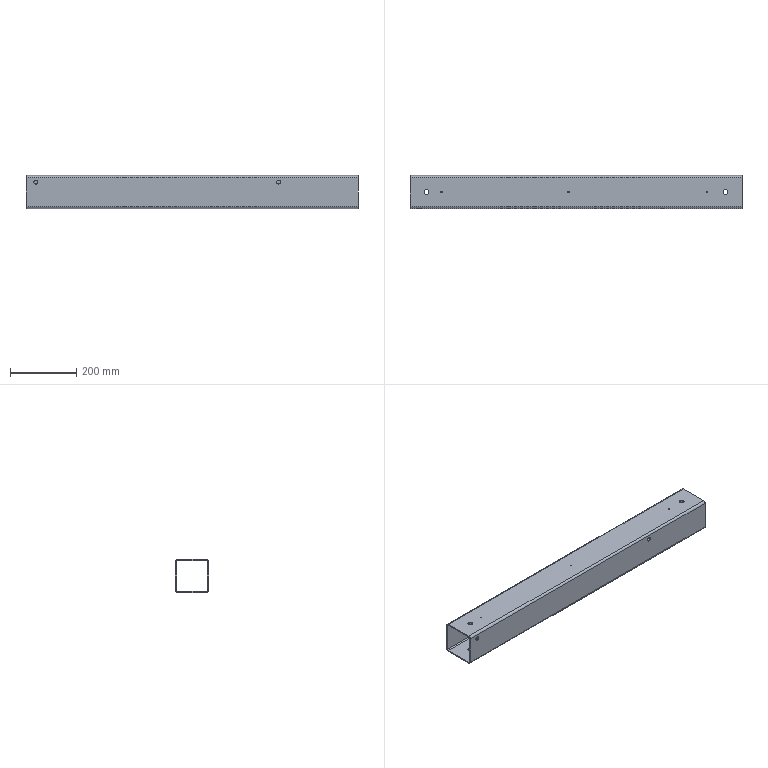Part | STEP file | [04] | 1 solid | 40 faces | box 1005 x 100 x 100 mm | volume 1215446 mm3 | cylinder 30 | plane 10 | commonest cylinder face diameters 15 x8 4 x6 6 x4 6.4 x4 12 x4 12.8 x4